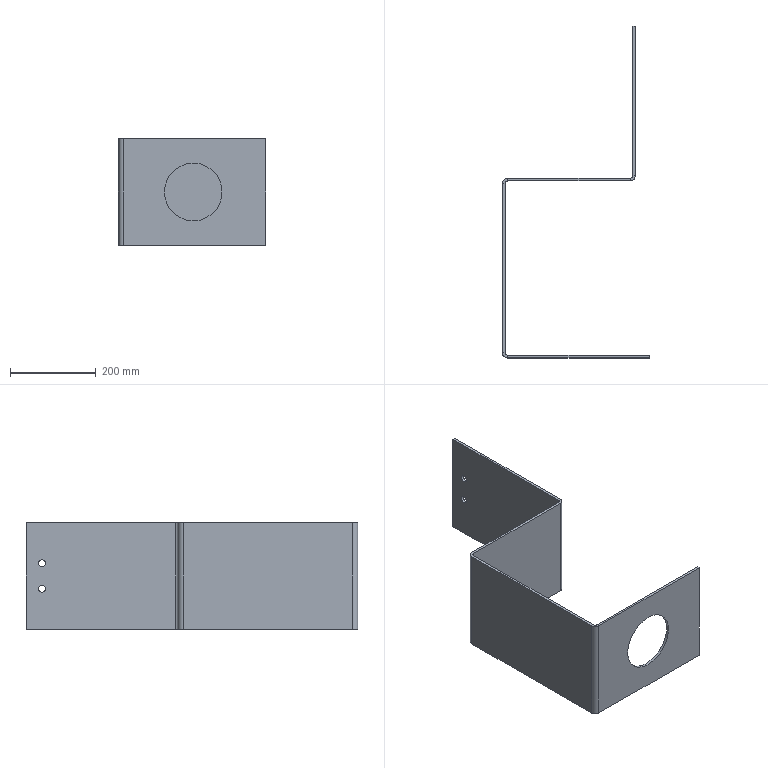Part | SolidWorks | features ICE 2, FlatPattern 1, SMBaseFlange 1, SheetMetal 1 | 1 solid | 36 faces | box 344 x 776 x 250 mm | volume 2022821 mm3 | plane 24 | cylinder 12 | commonest cylinder face diameters 16 x4 12 x3 24 x3 135 x2
STEP:
#1=CARTESIAN_POINT('',(-169.,6.,67.5));
#2=VERTEX_POINT('',#1);
#3=CARTESIAN_POINT('',(-169.,6.,-67.5));
#4=VERTEX_POINT('',#3);
#5=CARTESIAN_POINT('',(-169.,6.,0.));
#6=DIRECTION('',(0.,-1.,0.));
#7=DIRECTION('',(0.,0.,-1.));
#8=AXIS2_PLACEMENT_3D('',#5,#6,#7);
#9=CIRCLE('',#8,67.5);
#10=EDGE_CURVE('',#2,#4,#9,.T.);
#11=ORIENTED_EDGE('',*,*,#10,.F.);
#12=CARTESIAN_POINT('',(-169.,0.,67.5));
#13=VERTEX_POINT('',#12);
#14=CARTESIAN_POINT('',(-169.,6.,67.5));
#15=DIRECTION('',(0.,-1.,0.));
#16=VECTOR('',#15,1000.);
#17=LINE('',#14,#16);
#18=EDGE_CURVE('',#2,#13,#17,.T.);
#19=ORIENTED_EDGE('',*,*,#18,.T.);
#20=CARTESIAN_POINT('',(-169.,0.,-67.5));
#21=VERTEX_POINT('',#20);
#22=CARTESIAN_POINT('',(-169.,0.,0.));
#23=DIRECTION('',(0.,-1.,0.));
#24=DIRECTION('',(0.,0.,-1.));
#25=AXIS2_PLACEMENT_3D('',#22,#23,#24);
#26=CIRCLE('',#25,67.5);
#27=EDGE_CURVE('',#13,#21,#26,.T.);
#28=ORIENTED_EDGE('',*,*,#27,.T.);
#29=CARTESIAN_POINT('',(-169.,6.,-67.5));
#30=DIRECTION('',(0.,-1.,0.));
#31=VECTOR('',#30,1000.);
#32=LINE('',#29,#31);
#33=EDGE_CURVE('',#4,#21,#32,.T.);
#34=ORIENTED_EDGE('',*,*,#33,.F.);
#35=EDGE_LOOP('',(#11,#19,#28,#34));
#36=FACE_OUTER_BOUND('',#35,.T.);
#37=CARTESIAN_POINT('',(-169.,6.,0.));
#38=DIRECTION('',(0.,-1.,0.));
#39=DIRECTION('',(0.,0.,-1.));
#40=AXIS2_PLACEMENT_3D('',#37,#38,#39);
#41=CYLINDRICAL_SURFACE('',#40,67.5);
#42=ADVANCED_FACE('',(#36),#41,.F.);
#43=CARTESIAN_POINT('',(-33.,739.,-38.));
#44=VERTEX_POINT('',#43);
#45=CARTESIAN_POINT('',(-33.,739.,-22.));
#46=VERTEX_POINT('',#45);
#47=CARTESIAN_POINT('',(-33.,739.,-30.));
#48=DIRECTION('',(-1.,0.,0.));
#49=DIRECTION('',(0.,0.,1.));
#50=AXIS2_PLACEMENT_3D('',#47,#48,#49);
#51=CIRCLE('',#50,8.);
#52=EDGE_CURVE('',#44,#46,#51,.T.);
#53=ORIENTED_EDGE('',*,*,#52,.F.);
#54=CARTESIAN_POINT('',(-39.,739.,-38.));
#55=VERTEX_POINT('',#54);
#56=CARTESIAN_POINT('',(-33.,739.,-38.));
#57=DIRECTION('',(-1.,0.,0.));
#58=VECTOR('',#57,1000.);
#59=LINE('',#56,#58);
#60=EDGE_CURVE('',#44,#55,#59,.T.);
#61=ORIENTED_EDGE('',*,*,#60,.T.);
#62=CARTESIAN_POINT('',(-39.,739.,-22.));
#63=VERTEX_POINT('',#62);
#64=CARTESIAN_POINT('',(-39.,739.,-30.));
#65=DIRECTION('',(-1.,0.,0.));
#66=DIRECTION('',(0.,0.,1.));
#67=AXIS2_PLACEMENT_3D('',#64,#65,#66);
#68=CIRCLE('',#67,8.);
#69=EDGE_CURVE('',#55,#63,#68,.T.);
#70=ORIENTED_EDGE('',*,*,#69,.T.);
#71=CARTESIAN_POINT('',(-33.,739.,-22.));
#72=DIRECTION('',(-1.,0.,0.));
#73=VECTOR('',#72,1000.);
#74=LINE('',#71,#73);
#75=EDGE_CURVE('',#46,#63,#74,.T.);
#76=ORIENTED_EDGE('',*,*,#75,.F.);
#77=EDGE_LOOP('',(#53,#61,#70,#76));
#78=FACE_OUTER_BOUND('',#77,.T.);
#79=CARTESIAN_POINT('',(-33.,739.,-30.));
#80=DIRECTION('',(-1.,0.,0.));
#81=DIRECTION('',(0.,0.,1.));
#82=AXIS2_PLACEMENT_3D('',#79,#80,#81);
#83=CYLINDRICAL_SURFACE('',#82,8.);
#84=ADVANCED_FACE('',(#78),#83,.F.);
#85=CARTESIAN_POINT('',(-33.,739.,22.));
#86=VERTEX_POINT('',#85);
#87=CARTESIAN_POINT('',(-33.,739.,38.));
#88=VERTEX_POINT('',#87);
#89=CARTESIAN_POINT('',(-33.,739.,30.));
#90=DIRECTION('',(-1.,0.,0.));
#91=DIRECTION('',(0.,0.,1.));
#92=AXIS2_PLACEMENT_3D('',#89,#90,#91);
#93=CIRCLE('',#92,8.);
#94=EDGE_CURVE('',#86,#88,#93,.T.);
#95=ORIENTED_EDGE('',*,*,#94,.F.);
#96=CARTESIAN_POINT('',(-39.,739.,22.));
#97=VERTEX_POINT('',#96);
#98=CARTESIAN_POINT('',(-33.,739.,22.));
#99=DIRECTION('',(-1.,0.,0.));
#100=VECTOR('',#99,1000.);
#101=LINE('',#98,#100);
#102=EDGE_CURVE('',#86,#97,#101,.T.);
#103=ORIENTED_EDGE('',*,*,#102,.T.);
#104=CARTESIAN_POINT('',(-39.,739.,38.));
#105=VERTEX_POINT('',#104);
#106=CARTESIAN_POINT('',(-39.,739.,30.));
#107=DIRECTION('',(-1.,0.,0.));
#108=DIRECTION('',(0.,0.,1.));
#109=AXIS2_PLACEMENT_3D('',#106,#107,#108);
#110=CIRCLE('',#109,8.);
#111=EDGE_CURVE('',#97,#105,#110,.T.);
#112=ORIENTED_EDGE('',*,*,#111,.T.);
#113=CARTESIAN_POINT('',(-33.,739.,38.));
#114=DIRECTION('',(-1.,0.,0.));
#115=VECTOR('',#114,1000.);
#116=LINE('',#113,#115);
#117=EDGE_CURVE('',#88,#105,#116,.T.);
#118=ORIENTED_EDGE('',*,*,#117,.F.);
#119=EDGE_LOOP('',(#95,#103,#112,#118));
#120=FACE_OUTER_BOUND('',#119,.T.);
#121=CARTESIAN_POINT('',(-33.,739.,30.));
#122=DIRECTION('',(-1.,0.,0.));
#123=DIRECTION('',(0.,0.,1.));
#124=AXIS2_PLACEMENT_3D('',#121,#122,#123);
#125=CYLINDRICAL_SURFACE('',#124,8.);
#126=ADVANCED_FACE('',(#120),#125,.F.);
#127=CARTESIAN_POINT('',(-344.,12.,125.));
#128=VERTEX_POINT('',#127);
#129=CARTESIAN_POINT('',(-338.,12.,125.));
#130=VERTEX_POINT('',#129);
#131=CARTESIAN_POINT('',(-344.,12.,125.));
#132=DIRECTION('',(1.,0.,0.));
#133=VECTOR('',#132,1000.);
#134=LINE('',#131,#133);
#135=EDGE_CURVE('',#128,#130,#134,.T.);
#136=ORIENTED_EDGE('',*,*,#135,.F.);
#137=CARTESIAN_POINT('',(-332.,0.,125.));
#138=VERTEX_POINT('',#137);
#139=CARTESIAN_POINT('',(-332.,12.,125.));
#140=DIRECTION('',(0.,0.,-1.));
#141=DIRECTION('',(1.,0.,0.));
#142=AXIS2_PLACEMENT_3D('',#139,#140,#141);
#143=CIRCLE('',#142,12.);
#144=EDGE_CURVE('',#138,#128,#143,.T.);
#145=ORIENTED_EDGE('',*,*,#144,.F.);
#146=CARTESIAN_POINT('',(-332.,6.,125.));
#147=VERTEX_POINT('',#146);
#148=CARTESIAN_POINT('',(-332.,6.,125.));
#149=DIRECTION('',(0.,-1.,0.));
#150=VECTOR('',#149,1000.);
#151=LINE('',#148,#150);
#152=EDGE_CURVE('',#147,#138,#151,.T.);
#153=ORIENTED_EDGE('',*,*,#152,.F.);
#154=CARTESIAN_POINT('',(-332.,12.,125.));
#155=DIRECTION('',(0.,0.,-1.));
#156=DIRECTION('',(1.,0.,0.));
#157=AXIS2_PLACEMENT_3D('',#154,#155,#156);
#158=CIRCLE('',#157,6.);
#159=EDGE_CURVE('',#147,#130,#158,.T.);
#160=ORIENTED_EDGE('',*,*,#159,.T.);
#161=EDGE_LOOP('',(#136,#145,#153,#160));
#162=FACE_OUTER_BOUND('',#161,.T.);
#163=CARTESIAN_POINT('',(-344.,12.,125.));
#164=DIRECTION('',(0.,0.,1.));
#165=DIRECTION('',(1.,0.,0.));
#166=AXIS2_PLACEMENT_3D('',#163,#164,#165);
#167=PLANE('',#166);
#168=ADVANCED_FACE('',(#162),#167,.T.);
#169=CARTESIAN_POINT('',(-344.,408.,125.));
#170=VERTEX_POINT('',#169);
#171=CARTESIAN_POINT('',(-344.,0.,125.));
#172=DIRECTION('',(0.,1.,0.));
#173=VECTOR('',#172,1000.);
#174=LINE('',#171,#173);
#175=EDGE_CURVE('',#128,#170,#174,.T.);
#176=ORIENTED_EDGE('',*,*,#175,.F.);
#177=ORIENTED_EDGE('',*,*,#135,.T.);
#178=CARTESIAN_POINT('',(-338.,408.,125.));
#179=VERTEX_POINT('',#178);
#180=CARTESIAN_POINT('',(-338.,0.,125.));
#181=DIRECTION('',(0.,1.,0.));
#182=VECTOR('',#181,1000.);
#183=LINE('',#180,#182);
#184=EDGE_CURVE('',#130,#179,#183,.T.);
#185=ORIENTED_EDGE('',*,*,#184,.T.);
#186=CARTESIAN_POINT('',(-338.,408.,125.));
#187=DIRECTION('',(-1.,0.,0.));
#188=VECTOR('',#187,1000.);
#189=LINE('',#186,#188);
#190=EDGE_CURVE('',#179,#170,#189,.T.);
#191=ORIENTED_EDGE('',*,*,#190,.T.);
#192=EDGE_LOOP('',(#176,#177,#185,#191));
#193=FACE_OUTER_BOUND('',#192,.T.);
#194=CARTESIAN_POINT('',(-332.,6.,125.));
#195=DIRECTION('',(0.,0.,1.));
#196=DIRECTION('',(1.,0.,0.));
#197=AXIS2_PLACEMENT_3D('',#194,#195,#196);
#198=PLANE('',#197);
#199=ADVANCED_FACE('',(#193),#198,.T.);
#200=CARTESIAN_POINT('',(-332.,0.,-125.));
#201=VERTEX_POINT('',#200);
#202=CARTESIAN_POINT('',(-332.,6.,-125.));
#203=VERTEX_POINT('',#202);
#204=CARTESIAN_POINT('',(-332.,0.,-125.));
#205=DIRECTION('',(0.,1.,0.));
#206=VECTOR('',#205,1000.);
#207=LINE('',#204,#206);
#208=EDGE_CURVE('',#201,#203,#207,.T.);
#209=ORIENTED_EDGE('',*,*,#208,.F.);
#210=CARTESIAN_POINT('',(-344.,12.,-125.));
#211=VERTEX_POINT('',#210);
#212=CARTESIAN_POINT('',(-332.,12.,-125.));
#213=DIRECTION('',(0.,0.,-1.));
#214=DIRECTION('',(1.,0.,0.));
#215=AXIS2_PLACEMENT_3D('',#212,#213,#214);
#216=CIRCLE('',#215,12.);
#217=EDGE_CURVE('',#201,#211,#216,.T.);
#218=ORIENTED_EDGE('',*,*,#217,.T.);
#219=CARTESIAN_POINT('',(-338.,12.,-125.));
#220=VERTEX_POINT('',#219);
#221=CARTESIAN_POINT('',(-338.,12.,-125.));
#222=DIRECTION('',(-1.,0.,0.));
#223=VECTOR('',#222,1000.);
#224=LINE('',#221,#223);
#225=EDGE_CURVE('',#220,#211,#224,.T.);
#226=ORIENTED_EDGE('',*,*,#225,.F.);
#227=CARTESIAN_POINT('',(-332.,12.,-125.));
#228=DIRECTION('',(0.,0.,-1.));
#229=DIRECTION('',(1.,0.,0.));
#230=AXIS2_PLACEMENT_3D('',#227,#228,#229);
#231=CIRCLE('',#230,6.);
#232=EDGE_CURVE('',#203,#220,#231,.T.);
#233=ORIENTED_EDGE('',*,*,#232,.F.);
#234=EDGE_LOOP('',(#209,#218,#226,#233));
#235=FACE_OUTER_BOUND('',#234,.T.);
#236=CARTESIAN_POINT('',(-332.,0.,-125.));
#237=DIRECTION('',(0.,0.,-1.));
#238=DIRECTION('',(-1.,0.,0.));
#239=AXIS2_PLACEMENT_3D('',#236,#237,#238);
#240=PLANE('',#239);
#241=ADVANCED_FACE('',(#235),#240,.T.);
#242=CARTESIAN_POINT('',(0.,0.,-125.));
#243=VERTEX_POINT('',#242);
#244=CARTESIAN_POINT('',(0.,0.,-125.));
#245=DIRECTION('',(-1.,0.,0.));
#246=VECTOR('',#245,1000.);
#247=LINE('',#244,#246);
#248=EDGE_CURVE('',#243,#201,#247,.T.);
#249=ORIENTED_EDGE('',*,*,#248,.T.);
#250=ORIENTED_EDGE('',*,*,#208,.T.);
#251=CARTESIAN_POINT('',(0.,6.,-125.));
#252=VERTEX_POINT('',#251);
#253=CARTESIAN_POINT('',(0.,6.,-125.));
#254=DIRECTION('',(-1.,0.,0.));
#255=VECTOR('',#254,1000.);
#256=LINE('',#253,#255);
#257=EDGE_CURVE('',#252,#203,#256,.T.);
#258=ORIENTED_EDGE('',*,*,#257,.F.);
#259=CARTESIAN_POINT('',(0.,6.,-125.));
#260=DIRECTION('',(0.,-1.,0.));
#261=VECTOR('',#260,1000.);
#262=LINE('',#259,#261);
#263=EDGE_CURVE('',#252,#243,#262,.T.);
#264=ORIENTED_EDGE('',*,*,#263,.T.);
#265=EDGE_LOOP('',(#249,#250,#258,#264));
#266=FACE_OUTER_BOUND('',#265,.T.);
#267=CARTESIAN_POINT('',(-338.,12.,-125.));
#268=DIRECTION('',(0.,0.,-1.));
#269=DIRECTION('',(-1.,0.,0.));
#270=AXIS2_PLACEMENT_3D('',#267,#268,#269);
#271=PLANE('',#270);
#272=ADVANCED_FACE('',(#266),#271,.T.);
#273=CARTESIAN_POINT('',(-332.,420.,125.));
#274=VERTEX_POINT('',#273);
#275=CARTESIAN_POINT('',(-332.,414.,125.));
#276=VERTEX_POINT('',#275);
#277=CARTESIAN_POINT('',(-332.,420.,125.));
#278=DIRECTION('',(0.,-1.,0.));
#279=VECTOR('',#278,1000.);
#280=LINE('',#277,#279);
#281=EDGE_CURVE('',#274,#276,#280,.T.);
#282=ORIENTED_EDGE('',*,*,#281,.F.);
#283=CARTESIAN_POINT('',(-332.,408.,125.));
#284=DIRECTION('',(0.,0.,-1.));
#285=DIRECTION('',(1.,0.,0.));
#286=AXIS2_PLACEMENT_3D('',#283,#284,#285);
#287=CIRCLE('',#286,12.);
#288=EDGE_CURVE('',#170,#274,#287,.T.);
#289=ORIENTED_EDGE('',*,*,#288,.F.);
#290=ORIENTED_EDGE('',*,*,#190,.F.);
#291=CARTESIAN_POINT('',(-332.,408.,125.));
#292=DIRECTION('',(0.,0.,-1.));
#293=DIRECTION('',(1.,0.,0.));
#294=AXIS2_PLACEMENT_3D('',#291,#292,#293);
#295=CIRCLE('',#294,6.);
#296=EDGE_CURVE('',#179,#276,#295,.T.);
#297=ORIENTED_EDGE('',*,*,#296,.T.);
#298=EDGE_LOOP('',(#282,#289,#290,#297));
#299=FACE_OUTER_BOUND('',#298,.T.);
#300=CARTESIAN_POINT('',(-332.,420.,125.));
#301=DIRECTION('',(0.,0.,1.));
#302=DIRECTION('',(1.,0.,0.));
#303=AXIS2_PLACEMENT_3D('',#300,#301,#302);
#304=PLANE('',#303);
#305=ADVANCED_FACE('',(#299),#304,.T.);
#306=CARTESIAN_POINT('',(-45.,420.,125.));
#307=VERTEX_POINT('',#306);
#308=CARTESIAN_POINT('',(-344.,420.,125.));
#309=DIRECTION('',(1.,0.,0.));
#310=VECTOR('',#309,1000.);
#311=LINE('',#308,#310);
#312=EDGE_CURVE('',#274,#307,#311,.T.);
#313=ORIENTED_EDGE('',*,*,#312,.F.);
#314=ORIENTED_EDGE('',*,*,#281,.T.);
#315=CARTESIAN_POINT('',(-45.,414.,125.));
#316=VERTEX_POINT('',#315);
#317=CARTESIAN_POINT('',(-344.,414.,125.));
#318=DIRECTION('',(1.,0.,0.));
#319=VECTOR('',#318,1000.);
#320=LINE('',#317,#319);
#321=EDGE_CURVE('',#276,#316,#320,.T.);
#322=ORIENTED_EDGE('',*,*,#321,.T.);
#323=CARTESIAN_POINT('',(-45.,414.,125.));
#324=DIRECTION('',(0.,1.,0.));
#325=VECTOR('',#324,1000.);
#326=LINE('',#323,#325);
#327=EDGE_CURVE('',#316,#307,#326,.T.);
#328=ORIENTED_EDGE('',*,*,#327,.T.);
#329=EDGE_LOOP('',(#313,#314,#322,#328));
#330=FACE_OUTER_BOUND('',#329,.T.);
#331=CARTESIAN_POINT('',(-338.,408.,125.));
#332=DIRECTION('',(0.,0.,1.));
#333=DIRECTION('',(1.,0.,0.));
#334=AXIS2_PLACEMENT_3D('',#331,#332,#333);
#335=PLANE('',#334);
#336=ADVANCED_FACE('',(#330),#335,.T.);
#337=CARTESIAN_POINT('',(-344.,408.,-125.));
#338=VERTEX_POINT('',#337);
#339=CARTESIAN_POINT('',(-338.,408.,-125.));
#340=VERTEX_POINT('',#339);
#341=CARTESIAN_POINT('',(-344.,408.,-125.));
#342=DIRECTION('',(1.,0.,0.));
#343=VECTOR('',#342,1000.);
#344=LINE('',#341,#343);
#345=EDGE_CURVE('',#338,#340,#344,.T.);
#346=ORIENTED_EDGE('',*,*,#345,.F.);
#347=CARTESIAN_POINT('',(-332.,420.,-125.));
#348=VERTEX_POINT('',#347);
#349=CARTESIAN_POINT('',(-332.,408.,-125.));
#350=DIRECTION('',(0.,0.,-1.));
#351=DIRECTION('',(1.,0.,0.));
#352=AXIS2_PLACEMENT_3D('',#349,#350,#351);
#353=CIRCLE('',#352,12.);
#354=EDGE_CURVE('',#338,#348,#353,.T.);
#355=ORIENTED_EDGE('',*,*,#354,.T.);
#356=CARTESIAN_POINT('',(-332.,414.,-125.));
#357=VERTEX_POINT('',#356);
#358=CARTESIAN_POINT('',(-332.,414.,-125.));
#359=DIRECTION('',(0.,1.,0.));
#360=VECTOR('',#359,1000.);
#361=LINE('',#358,#360);
#362=EDGE_CURVE('',#357,#348,#361,.T.);
#363=ORIENTED_EDGE('',*,*,#362,.F.);
#364=CARTESIAN_POINT('',(-332.,408.,-125.));
#365=DIRECTION('',(0.,0.,-1.));
#366=DIRECTION('',(1.,0.,0.));
#367=AXIS2_PLACEMENT_3D('',#364,#365,#366);
#368=CIRCLE('',#367,6.);
#369=EDGE_CURVE('',#340,#357,#368,.T.);
#370=ORIENTED_EDGE('',*,*,#369,.F.);
#371=EDGE_LOOP('',(#346,#355,#363,#370));
#372=FACE_OUTER_BOUND('',#371,.T.);
#373=CARTESIAN_POINT('',(-344.,408.,-125.));
#374=DIRECTION('',(0.,0.,-1.));
#375=DIRECTION('',(-1.,0.,0.));
#376=AXIS2_PLACEMENT_3D('',#373,#374,#375);
#377=PLANE('',#376);
#378=ADVANCED_FACE('',(#372),#377,.T.);
#379=CARTESIAN_POINT('',(-344.,0.,-125.));
#380=DIRECTION('',(0.,1.,0.));
#381=VECTOR('',#380,1000.);
#382=LINE('',#379,#381);
#383=EDGE_CURVE('',#211,#338,#382,.T.);
#384=ORIENTED_EDGE('',*,*,#383,.T.);
#385=ORIENTED_EDGE('',*,*,#345,.T.);
#386=CARTESIAN_POINT('',(-338.,0.,-125.));
#387=DIRECTION('',(0.,1.,0.));
#388=VECTOR('',#387,1000.);
#389=LINE('',#386,#388);
#390=EDGE_CURVE('',#220,#340,#389,.T.);
#391=ORIENTED_EDGE('',*,*,#390,.F.);
#392=ORIENTED_EDGE('',*,*,#225,.T.);
#393=EDGE_LOOP('',(#384,#385,#391,#392));
#394=FACE_OUTER_BOUND('',#393,.T.);
#395=CARTESIAN_POINT('',(-332.,414.,-125.));
#396=DIRECTION('',(0.,0.,-1.));
#397=DIRECTION('',(-1.,0.,0.));
#398=AXIS2_PLACEMENT_3D('',#395,#396,#397);
#399=PLANE('',#398);
#400=ADVANCED_FACE('',(#394),#399,.T.);
#401=CARTESIAN_POINT('',(-39.,426.,125.));
#402=VERTEX_POINT('',#401);
#403=CARTESIAN_POINT('',(-33.,426.,125.));
#404=VERTEX_POINT('',#403);
#405=CARTESIAN_POINT('',(-39.,426.,125.));
#406=DIRECTION('',(1.,0.,0.));
#407=VECTOR('',#406,1000.);
#408=LINE('',#405,#407);
#409=EDGE_CURVE('',#402,#404,#408,.T.);
#410=ORIENTED_EDGE('',*,*,#409,.F.);
#411=CARTESIAN_POINT('',(-45.,426.,125.));
#412=DIRECTION('',(0.,0.,1.));
#413=DIRECTION('',(-1.,0.,0.));
#414=AXIS2_PLACEMENT_3D('',#411,#412,#413);
#415=CIRCLE('',#414,6.);
#416=EDGE_CURVE('',#307,#402,#415,.T.);
#417=ORIENTED_EDGE('',*,*,#416,.F.);
#418=ORIENTED_EDGE('',*,*,#327,.F.);
#419=CARTESIAN_POINT('',(-45.,426.,125.));
#420=DIRECTION('',(0.,0.,1.));
#421=DIRECTION('',(1.,0.,0.));
#422=AXIS2_PLACEMENT_3D('',#419,#420,#421);
#423=CIRCLE('',#422,12.);
#424=EDGE_CURVE('',#316,#404,#423,.T.);
#425=ORIENTED_EDGE('',*,*,#424,.T.);
#426=EDGE_LOOP('',(#410,#417,#418,#425));
#427=FACE_OUTER_BOUND('',#426,.T.);
#428=CARTESIAN_POINT('',(-39.,426.,125.));
#429=DIRECTION('',(0.,0.,1.));
#430=DIRECTION('',(1.,0.,0.));
#431=AXIS2_PLACEMENT_3D('',#428,#429,#430);
#432=PLANE('',#431);
#433=ADVANCED_FACE('',(#427),#432,.T.);
#434=CARTESIAN_POINT('',(-39.,776.,125.));
#435=VERTEX_POINT('',#434);
#436=CARTESIAN_POINT('',(-39.,420.,125.));
#437=DIRECTION('',(0.,1.,0.));
#438=VECTOR('',#437,1000.);
#439=LINE('',#436,#438);
#440=EDGE_CURVE('',#402,#435,#439,.T.);
#441=ORIENTED_EDGE('',*,*,#440,.F.);
#442=ORIENTED_EDGE('',*,*,#409,.T.);
#443=CARTESIAN_POINT('',(-33.,776.,125.));
#444=VERTEX_POINT('',#443);
#445=CARTESIAN_POINT('',(-33.,420.,125.));
#446=DIRECTION('',(0.,1.,0.));
#447=VECTOR('',#446,1000.);
#448=LINE('',#445,#447);
#449=EDGE_CURVE('',#404,#444,#448,.T.);
#450=ORIENTED_EDGE('',*,*,#449,.T.);
#451=CARTESIAN_POINT('',(-39.,776.,125.));
#452=DIRECTION('',(1.,0.,0.));
#453=VECTOR('',#452,1000.);
#454=LINE('',#451,#453);
#455=EDGE_CURVE('',#435,#444,#454,.T.);
#456=ORIENTED_EDGE('',*,*,#455,.F.);
#457=EDGE_LOOP('',(#441,#442,#450,#456));
#458=FACE_OUTER_BOUND('',#457,.T.);
#459=CARTESIAN_POINT('',(-45.,414.,125.));
#460=DIRECTION('',(0.,0.,1.));
#461=DIRECTION('',(1.,0.,0.));
#462=AXIS2_PLACEMENT_3D('',#459,#460,#461);
#463=PLANE('',#462);
#464=ADVANCED_FACE('',(#458),#463,.T.);
#465=CARTESIAN_POINT('',(-45.,420.,-125.));
#466=VERTEX_POINT('',#465);
#467=CARTESIAN_POINT('',(-45.,414.,-125.));
#468=VERTEX_POINT('',#467);
#469=CARTESIAN_POINT('',(-45.,420.,-125.));
#470=DIRECTION('',(0.,-1.,0.));
#471=VECTOR('',#470,1000.);
#472=LINE('',#469,#471);
#473=EDGE_CURVE('',#466,#468,#472,.T.);
#474=ORIENTED_EDGE('',*,*,#473,.F.);
#475=CARTESIAN_POINT('',(-39.,426.,-125.));
#476=VERTEX_POINT('',#475);
#477=CARTESIAN_POINT('',(-45.,426.,-125.));
#478=DIRECTION('',(0.,0.,1.));
#479=DIRECTION('',(-1.,0.,0.));
#480=AXIS2_PLACEMENT_3D('',#477,#478,#479);
#481=CIRCLE('',#480,6.);
#482=EDGE_CURVE('',#466,#476,#481,.T.);
#483=ORIENTED_EDGE('',*,*,#482,.T.);
#484=CARTESIAN_POINT('',(-33.,426.,-125.));
#485=VERTEX_POINT('',#484);
#486=CARTESIAN_POINT('',(-33.,426.,-125.));
#487=DIRECTION('',(-1.,0.,0.));
#488=VECTOR('',#487,1000.);
#489=LINE('',#486,#488);
#490=EDGE_CURVE('',#485,#476,#489,.T.);
#491=ORIENTED_EDGE('',*,*,#490,.F.);
#492=CARTESIAN_POINT('',(-45.,426.,-125.));
#493=DIRECTION('',(0.,0.,1.));
#494=DIRECTION('',(1.,0.,0.));
#495=AXIS2_PLACEMENT_3D('',#492,#493,#494);
#496=CIRCLE('',#495,12.);
#497=EDGE_CURVE('',#468,#485,#496,.T.);
#498=ORIENTED_EDGE('',*,*,#497,.F.);
#499=EDGE_LOOP('',(#474,#483,#491,#498));
#500=FACE_OUTER_BOUND('',#499,.T.);
#501=CARTESIAN_POINT('',(-45.,420.,-125.));
#502=DIRECTION('',(0.,0.,-1.));
#503=DIRECTION('',(-1.,0.,0.));
#504=AXIS2_PLACEMENT_3D('',#501,#502,#503);
#505=PLANE('',#504);
#506=ADVANCED_FACE('',(#500),#505,.T.);
#507=CARTESIAN_POINT('',(-344.,420.,-125.));
#508=DIRECTION('',(1.,0.,0.));
#509=VECTOR('',#508,1000.);
#510=LINE('',#507,#509);
#511=EDGE_CURVE('',#348,#466,#510,.T.);
#512=ORIENTED_EDGE('',*,*,#511,.T.);
#513=ORIENTED_EDGE('',*,*,#473,.T.);
#514=CARTESIAN_POINT('',(-344.,414.,-125.));
#515=DIRECTION('',(1.,0.,0.));
#516=VECTOR('',#515,1000.);
#517=LINE('',#514,#516);
#518=EDGE_CURVE('',#357,#468,#517,.T.);
#519=ORIENTED_EDGE('',*,*,#518,.F.);
#520=ORIENTED_EDGE('',*,*,#362,.T.);
#521=EDGE_LOOP('',(#512,#513,#519,#520));
#522=FACE_OUTER_BOUND('',#521,.T.);
#523=CARTESIAN_POINT('',(-33.,426.,-125.));
#524=DIRECTION('',(0.,0.,-1.));
#525=DIRECTION('',(-1.,0.,0.));
#526=AXIS2_PLACEMENT_3D('',#523,#524,#525);
#527=PLANE('',#526);
#528=ADVANCED_FACE('',(#522),#527,.T.);
#529=CARTESIAN_POINT('',(-33.,739.,-30.));
#530=DIRECTION('',(-1.,0.,0.));
#531=DIRECTION('',(0.,0.,1.));
#532=AXIS2_PLACEMENT_3D('',#529,#530,#531);
#533=CIRCLE('',#532,8.);
#534=EDGE_CURVE('',#46,#44,#533,.T.);
#535=ORIENTED_EDGE('',*,*,#534,.T.);
#536=ORIENTED_EDGE('',*,*,#52,.T.);
#537=EDGE_LOOP('',(#535,#536));
#538=FACE_BOUND('',#537,.T.);
#539=CARTESIAN_POINT('',(-33.,739.,30.));
#540=DIRECTION('',(-1.,0.,0.));
#541=DIRECTION('',(0.,0.,1.));
#542=AXIS2_PLACEMENT_3D('',#539,#540,#541);
#543=CIRCLE('',#542,8.);
#544=EDGE_CURVE('',#88,#86,#543,.T.);
#545=ORIENTED_EDGE('',*,*,#544,.T.);
#546=ORIENTED_EDGE('',*,*,#94,.T.);
#547=EDGE_LOOP('',(#545,#546));
#548=FACE_BOUND('',#547,.T.);
#549=CARTESIAN_POINT('',(-33.,776.,-125.));
#550=VERTEX_POINT('',#549);
#551=CARTESIAN_POINT('',(-33.,420.,-125.));
#552=DIRECTION('',(0.,1.,0.));
#553=VECTOR('',#552,1000.);
#554=LINE('',#551,#553);
#555=EDGE_CURVE('',#485,#550,#554,.T.);
#556=ORIENTED_EDGE('',*,*,#555,.T.);
#557=CARTESIAN_POINT('',(-33.,776.,125.));
#558=DIRECTION('',(0.,0.,-1.));
#559=VECTOR('',#558,1000.);
#560=LINE('',#557,#559);
#561=EDGE_CURVE('',#444,#550,#560,.T.);
#562=ORIENTED_EDGE('',*,*,#561,.F.);
#563=ORIENTED_EDGE('',*,*,#449,.F.);
#564=CARTESIAN_POINT('',(-33.,426.,125.));
#565=DIRECTION('',(0.,0.,-1.));
#566=VECTOR('',#565,1000.);
#567=LINE('',#564,#566);
#568=EDGE_CURVE('',#404,#485,#567,.T.);
#569=ORIENTED_EDGE('',*,*,#568,.T.);
#570=EDGE_LOOP('',(#556,#562,#563,#569));
#571=FACE_OUTER_BOUND('',#570,.T.);
#572=CARTESIAN_POINT('',(-33.,420.,125.));
#573=DIRECTION('',(-1.,0.,0.));
#574=DIRECTION('',(0.,0.,1.));
#575=AXIS2_PLACEMENT_3D('',#572,#573,#574);
#576=PLANE('',#575);
#577=ADVANCED_FACE('',(#538,#548,#571),#576,.F.);
#578=CARTESIAN_POINT('',(-39.,776.,-125.));
#579=VERTEX_POINT('',#578);
#580=CARTESIAN_POINT('',(-39.,776.,-125.));
#581=DIRECTION('',(1.,0.,0.));
#582=VECTOR('',#581,1000.);
#583=LINE('',#580,#582);
#584=EDGE_CURVE('',#579,#550,#583,.T.);
#585=ORIENTED_EDGE('',*,*,#584,.F.);
#586=CARTESIAN_POINT('',(-39.,776.,125.));
#587=DIRECTION('',(0.,0.,-1.));
#588=VECTOR('',#587,1000.);
#589=LINE('',#586,#588);
#590=EDGE_CURVE('',#435,#579,#589,.T.);
#591=ORIENTED_EDGE('',*,*,#590,.F.);
#592=ORIENTED_EDGE('',*,*,#455,.T.);
#593=ORIENTED_EDGE('',*,*,#561,.T.);
#594=EDGE_LOOP('',(#585,#591,#592,#593));
#595=FACE_OUTER_BOUND('',#594,.T.);
#596=CARTESIAN_POINT('',(-39.,776.,125.));
#597=DIRECTION('',(0.,1.,0.));
#598=DIRECTION('',(0.,0.,1.));
#599=AXIS2_PLACEMENT_3D('',#596,#597,#598);
#600=PLANE('',#599);
#601=ADVANCED_FACE('',(#595),#600,.T.);
#602=CARTESIAN_POINT('',(-39.,739.,-30.));
#603=DIRECTION('',(-1.,0.,0.));
#604=DIRECTION('',(0.,0.,1.));
#605=AXIS2_PLACEMENT_3D('',#602,#603,#604);
#606=CIRCLE('',#605,8.);
#607=EDGE_CURVE('',#63,#55,#606,.T.);
#608=ORIENTED_EDGE('',*,*,#607,.F.);
#609=ORIENTED_EDGE('',*,*,#69,.F.);
#610=EDGE_LOOP('',(#608,#609));
#611=FACE_BOUND('',#610,.T.);
#612=CARTESIAN_POINT('',(-39.,739.,30.));
#613=DIRECTION('',(-1.,0.,0.));
#614=DIRECTION('',(0.,0.,1.));
#615=AXIS2_PLACEMENT_3D('',#612,#613,#614);
#616=CIRCLE('',#615,8.);
#617=EDGE_CURVE('',#105,#97,#616,.T.);
#618=ORIENTED_EDGE('',*,*,#617,.F.);
#619=ORIENTED_EDGE('',*,*,#111,.F.);
#620=EDGE_LOOP('',(#618,#619));
#621=FACE_BOUND('',#620,.T.);
#622=CARTESIAN_POINT('',(-39.,420.,-125.));
#623=DIRECTION('',(0.,1.,0.));
#624=VECTOR('',#623,1000.);
#625=LINE('',#622,#624);
#626=EDGE_CURVE('',#476,#579,#625,.T.);
#627=ORIENTED_EDGE('',*,*,#626,.F.);
#628=CARTESIAN_POINT('',(-39.,426.,125.));
#629=DIRECTION('',(0.,0.,-1.));
#630=VECTOR('',#629,1000.);
#631=LINE('',#628,#630);
#632=EDGE_CURVE('',#402,#476,#631,.T.);
#633=ORIENTED_EDGE('',*,*,#632,.F.);
#634=ORIENTED_EDGE('',*,*,#440,.T.);
#635=ORIENTED_EDGE('',*,*,#590,.T.);
#636=EDGE_LOOP('',(#627,#633,#634,#635));
#637=FACE_OUTER_BOUND('',#636,.T.);
#638=CARTESIAN_POINT('',(-39.,420.,125.));
#639=DIRECTION('',(-1.,0.,0.));
#640=DIRECTION('',(0.,0.,1.));
#641=AXIS2_PLACEMENT_3D('',#638,#639,#640);
#642=PLANE('',#641);
#643=ADVANCED_FACE('',(#611,#621,#637),#642,.T.);
#644=ORIENTED_EDGE('',*,*,#482,.F.);
#645=CARTESIAN_POINT('',(-45.,420.,125.));
#646=DIRECTION('',(0.,0.,-1.));
#647=VECTOR('',#646,1000.);
#648=LINE('',#645,#647);
#649=EDGE_CURVE('',#307,#466,#648,.T.);
#650=ORIENTED_EDGE('',*,*,#649,.F.);
#651=ORIENTED_EDGE('',*,*,#416,.T.);
#652=ORIENTED_EDGE('',*,*,#632,.T.);
#653=EDGE_LOOP('',(#644,#650,#651,#652));
#654=FACE_OUTER_BOUND('',#653,.T.);
#655=CARTESIAN_POINT('',(-45.,426.,125.));
#656=DIRECTION('',(0.,0.,-1.));
#657=DIRECTION('',(-1.,0.,0.));
#658=AXIS2_PLACEMENT_3D('',#655,#656,#657);
#659=CYLINDRICAL_SURFACE('',#658,6.);
#660=ADVANCED_FACE('',(#654),#659,.F.);
#661=ORIENTED_EDGE('',*,*,#511,.F.);
#662=CARTESIAN_POINT('',(-332.,420.,125.));
#663=DIRECTION('',(0.,0.,-1.));
#664=VECTOR('',#663,1000.);
#665=LINE('',#662,#664);
#666=EDGE_CURVE('',#274,#348,#665,.T.);
#667=ORIENTED_EDGE('',*,*,#666,.F.);
#668=ORIENTED_EDGE('',*,*,#312,.T.);
#669=ORIENTED_EDGE('',*,*,#649,.T.);
#670=EDGE_LOOP('',(#661,#667,#668,#669));
#671=FACE_OUTER_BOUND('',#670,.T.);
#672=CARTESIAN_POINT('',(-344.,420.,125.));
#673=DIRECTION('',(0.,1.,0.));
#674=DIRECTION('',(0.,0.,1.));
#675=AXIS2_PLACEMENT_3D('',#672,#673,#674);
#676=PLANE('',#675);
#677=ADVANCED_FACE('',(#671),#676,.T.);
#678=ORIENTED_EDGE('',*,*,#354,.F.);
#679=CARTESIAN_POINT('',(-344.,408.,125.));
#680=DIRECTION('',(0.,0.,-1.));
#681=VECTOR('',#680,1000.);
#682=LINE('',#679,#681);
#683=EDGE_CURVE('',#170,#338,#682,.T.);
#684=ORIENTED_EDGE('',*,*,#683,.F.);
#685=ORIENTED_EDGE('',*,*,#288,.T.);
#686=ORIENTED_EDGE('',*,*,#666,.T.);
#687=EDGE_LOOP('',(#678,#684,#685,#686));
#688=FACE_OUTER_BOUND('',#687,.T.);
#689=CARTESIAN_POINT('',(-332.,408.,125.));
#690=DIRECTION('',(0.,0.,-1.));
#691=DIRECTION('',(-1.,0.,0.));
#692=AXIS2_PLACEMENT_3D('',#689,#690,#691);
#693=CYLINDRICAL_SURFACE('',#692,12.);
#694=ADVANCED_FACE('',(#688),#693,.T.);
#695=ORIENTED_EDGE('',*,*,#383,.F.);
#696=CARTESIAN_POINT('',(-344.,12.,125.));
#697=DIRECTION('',(0.,0.,-1.));
#698=VECTOR('',#697,1000.);
#699=LINE('',#696,#698);
#700=EDGE_CURVE('',#128,#211,#699,.T.);
#701=ORIENTED_EDGE('',*,*,#700,.F.);
#702=ORIENTED_EDGE('',*,*,#175,.T.);
#703=ORIENTED_EDGE('',*,*,#683,.T.);
#704=EDGE_LOOP('',(#695,#701,#702,#703));
#705=FACE_OUTER_BOUND('',#704,.T.);
#706=CARTESIAN_POINT('',(-344.,0.,125.));
#707=DIRECTION('',(-1.,0.,0.));
#708=DIRECTION('',(0.,0.,1.));
#709=AXIS2_PLACEMENT_3D('',#706,#707,#708);
#710=PLANE('',#709);
#711=ADVANCED_FACE('',(#705),#710,.T.);
#712=ORIENTED_EDGE('',*,*,#217,.F.);
#713=CARTESIAN_POINT('',(-332.,0.,125.));
#714=DIRECTION('',(0.,0.,-1.));
#715=VECTOR('',#714,1000.);
#716=LINE('',#713,#715);
#717=EDGE_CURVE('',#138,#201,#716,.T.);
#718=ORIENTED_EDGE('',*,*,#717,.F.);
#719=ORIENTED_EDGE('',*,*,#144,.T.);
#720=ORIENTED_EDGE('',*,*,#700,.T.);
#721=EDGE_LOOP('',(#712,#718,#719,#720));
#722=FACE_OUTER_BOUND('',#721,.T.);
#723=CARTESIAN_POINT('',(-332.,12.,125.));
#724=DIRECTION('',(0.,0.,-1.));
#725=DIRECTION('',(-1.,0.,0.));
#726=AXIS2_PLACEMENT_3D('',#723,#724,#725);
#727=CYLINDRICAL_SURFACE('',#726,12.);
#728=ADVANCED_FACE('',(#722),#727,.T.);
#729=CARTESIAN_POINT('',(-169.,0.,0.));
#730=DIRECTION('',(0.,-1.,0.));
#731=DIRECTION('',(0.,0.,-1.));
#732=AXIS2_PLACEMENT_3D('',#729,#730,#731);
#733=CIRCLE('',#732,67.5);
#734=EDGE_CURVE('',#21,#13,#733,.T.);
#735=ORIENTED_EDGE('',*,*,#734,.F.);
#736=ORIENTED_EDGE('',*,*,#27,.F.);
#737=EDGE_LOOP('',(#735,#736));
#738=FACE_BOUND('',#737,.T.);
#739=ORIENTED_EDGE('',*,*,#248,.F.);
#740=CARTESIAN_POINT('',(0.,0.,125.));
#741=VERTEX_POINT('',#740);
#742=CARTESIAN_POINT('',(0.,0.,125.));
#743=DIRECTION('',(0.,0.,-1.));
#744=VECTOR('',#743,1000.);
#745=LINE('',#742,#744);
#746=EDGE_CURVE('',#741,#243,#745,.T.);
#747=ORIENTED_EDGE('',*,*,#746,.F.);
#748=CARTESIAN_POINT('',(0.,0.,125.));
#749=DIRECTION('',(-1.,0.,0.));
#750=VECTOR('',#749,1000.);
#751=LINE('',#748,#750);
#752=EDGE_CURVE('',#741,#138,#751,.T.);
#753=ORIENTED_EDGE('',*,*,#752,.T.);
#754=ORIENTED_EDGE('',*,*,#717,.T.);
#755=EDGE_LOOP('',(#739,#747,#753,#754));
#756=FACE_OUTER_BOUND('',#755,.T.);
#757=CARTESIAN_POINT('',(0.,0.,125.));
#758=DIRECTION('',(0.,-1.,0.));
#759=DIRECTION('',(0.,0.,-1.));
#760=AXIS2_PLACEMENT_3D('',#757,#758,#759);
#761=PLANE('',#760);
#762=ADVANCED_FACE('',(#738,#756),#761,.T.);
#763=ORIENTED_EDGE('',*,*,#263,.F.);
#764=CARTESIAN_POINT('',(0.,6.,125.));
#765=VERTEX_POINT('',#764);
#766=CARTESIAN_POINT('',(0.,6.,125.));
#767=DIRECTION('',(0.,0.,-1.));
#768=VECTOR('',#767,1000.);
#769=LINE('',#766,#768);
#770=EDGE_CURVE('',#765,#252,#769,.T.);
#771=ORIENTED_EDGE('',*,*,#770,.F.);
#772=CARTESIAN_POINT('',(0.,6.,125.));
#773=DIRECTION('',(0.,-1.,0.));
#774=VECTOR('',#773,1000.);
#775=LINE('',#772,#774);
#776=EDGE_CURVE('',#765,#741,#775,.T.);
#777=ORIENTED_EDGE('',*,*,#776,.T.);
#778=ORIENTED_EDGE('',*,*,#746,.T.);
#779=EDGE_LOOP('',(#763,#771,#777,#778));
#780=FACE_OUTER_BOUND('',#779,.T.);
#781=CARTESIAN_POINT('',(0.,6.,125.));
#782=DIRECTION('',(1.,0.,0.));
#783=DIRECTION('',(0.,0.,-1.));
#784=AXIS2_PLACEMENT_3D('',#781,#782,#783);
#785=PLANE('',#784);
#786=ADVANCED_FACE('',(#780),#785,.T.);
#787=CARTESIAN_POINT('',(-169.,6.,0.));
#788=DIRECTION('',(0.,-1.,0.));
#789=DIRECTION('',(0.,0.,-1.));
#790=AXIS2_PLACEMENT_3D('',#787,#788,#789);
#791=CIRCLE('',#790,67.5);
#792=EDGE_CURVE('',#4,#2,#791,.T.);
#793=ORIENTED_EDGE('',*,*,#792,.T.);
#794=ORIENTED_EDGE('',*,*,#10,.T.);
#795=EDGE_LOOP('',(#793,#794));
#796=FACE_BOUND('',#795,.T.);
#797=ORIENTED_EDGE('',*,*,#257,.T.);
#798=CARTESIAN_POINT('',(-332.,6.,125.));
#799=DIRECTION('',(0.,0.,-1.));
#800=VECTOR('',#799,1000.);
#801=LINE('',#798,#800);
#802=EDGE_CURVE('',#147,#203,#801,.T.);
#803=ORIENTED_EDGE('',*,*,#802,.F.);
#804=CARTESIAN_POINT('',(0.,6.,125.));
#805=DIRECTION('',(-1.,0.,0.));
#806=VECTOR('',#805,1000.);
#807=LINE('',#804,#806);
#808=EDGE_CURVE('',#765,#147,#807,.T.);
#809=ORIENTED_EDGE('',*,*,#808,.F.);
#810=ORIENTED_EDGE('',*,*,#770,.T.);
#811=EDGE_LOOP('',(#797,#803,#809,#810));
#812=FACE_OUTER_BOUND('',#811,.T.);
#813=CARTESIAN_POINT('',(0.,6.,125.));
#814=DIRECTION('',(0.,-1.,0.));
#815=DIRECTION('',(0.,0.,-1.));
#816=AXIS2_PLACEMENT_3D('',#813,#814,#815);
#817=PLANE('',#816);
#818=ADVANCED_FACE('',(#796,#812),#817,.F.);
#819=ORIENTED_EDGE('',*,*,#232,.T.);
#820=CARTESIAN_POINT('',(-338.,12.,125.));
#821=DIRECTION('',(0.,0.,-1.));
#822=VECTOR('',#821,1000.);
#823=LINE('',#820,#822);
#824=EDGE_CURVE('',#130,#220,#823,.T.);
#825=ORIENTED_EDGE('',*,*,#824,.F.);
#826=ORIENTED_EDGE('',*,*,#159,.F.);
#827=ORIENTED_EDGE('',*,*,#802,.T.);
#828=EDGE_LOOP('',(#819,#825,#826,#827));
#829=FACE_OUTER_BOUND('',#828,.T.);
#830=CARTESIAN_POINT('',(-332.,12.,125.));
#831=DIRECTION('',(0.,0.,-1.));
#832=DIRECTION('',(-1.,0.,0.));
#833=AXIS2_PLACEMENT_3D('',#830,#831,#832);
#834=CYLINDRICAL_SURFACE('',#833,6.);
#835=ADVANCED_FACE('',(#829),#834,.F.);
#836=ORIENTED_EDGE('',*,*,#390,.T.);
#837=CARTESIAN_POINT('',(-338.,408.,125.));
#838=DIRECTION('',(0.,0.,-1.));
#839=VECTOR('',#838,1000.);
#840=LINE('',#837,#839);
#841=EDGE_CURVE('',#179,#340,#840,.T.);
#842=ORIENTED_EDGE('',*,*,#841,.F.);
#843=ORIENTED_EDGE('',*,*,#184,.F.);
#844=ORIENTED_EDGE('',*,*,#824,.T.);
#845=EDGE_LOOP('',(#836,#842,#843,#844));
#846=FACE_OUTER_BOUND('',#845,.T.);
#847=CARTESIAN_POINT('',(-338.,0.,125.));
#848=DIRECTION('',(-1.,0.,0.));
#849=DIRECTION('',(0.,0.,1.));
#850=AXIS2_PLACEMENT_3D('',#847,#848,#849);
#851=PLANE('',#850);
#852=ADVANCED_FACE('',(#846),#851,.F.);
#853=ORIENTED_EDGE('',*,*,#369,.T.);
#854=CARTESIAN_POINT('',(-332.,414.,125.));
#855=DIRECTION('',(0.,0.,-1.));
#856=VECTOR('',#855,1000.);
#857=LINE('',#854,#856);
#858=EDGE_CURVE('',#276,#357,#857,.T.);
#859=ORIENTED_EDGE('',*,*,#858,.F.);
#860=ORIENTED_EDGE('',*,*,#296,.F.);
#861=ORIENTED_EDGE('',*,*,#841,.T.);
#862=EDGE_LOOP('',(#853,#859,#860,#861));
#863=FACE_OUTER_BOUND('',#862,.T.);
#864=CARTESIAN_POINT('',(-332.,408.,125.));
#865=DIRECTION('',(0.,0.,-1.));
#866=DIRECTION('',(-1.,0.,0.));
#867=AXIS2_PLACEMENT_3D('',#864,#865,#866);
#868=CYLINDRICAL_SURFACE('',#867,6.);
#869=ADVANCED_FACE('',(#863),#868,.F.);
#870=ORIENTED_EDGE('',*,*,#518,.T.);
#871=CARTESIAN_POINT('',(-45.,414.,125.));
#872=DIRECTION('',(0.,0.,-1.));
#873=VECTOR('',#872,1000.);
#874=LINE('',#871,#873);
#875=EDGE_CURVE('',#316,#468,#874,.T.);
#876=ORIENTED_EDGE('',*,*,#875,.F.);
#877=ORIENTED_EDGE('',*,*,#321,.F.);
#878=ORIENTED_EDGE('',*,*,#858,.T.);
#879=EDGE_LOOP('',(#870,#876,#877,#878));
#880=FACE_OUTER_BOUND('',#879,.T.);
#881=CARTESIAN_POINT('',(-344.,414.,125.));
#882=DIRECTION('',(0.,1.,0.));
#883=DIRECTION('',(0.,0.,1.));
#884=AXIS2_PLACEMENT_3D('',#881,#882,#883);
#885=PLANE('',#884);
#886=ADVANCED_FACE('',(#880),#885,.F.);
#887=ORIENTED_EDGE('',*,*,#497,.T.);
#888=ORIENTED_EDGE('',*,*,#568,.F.);
#889=ORIENTED_EDGE('',*,*,#424,.F.);
#890=ORIENTED_EDGE('',*,*,#875,.T.);
#891=EDGE_LOOP('',(#887,#888,#889,#890));
#892=FACE_OUTER_BOUND('',#891,.T.);
#893=CARTESIAN_POINT('',(-45.,426.,125.));
#894=DIRECTION('',(0.,0.,-1.));
#895=DIRECTION('',(-1.,0.,0.));
#896=AXIS2_PLACEMENT_3D('',#893,#894,#895);
#897=CYLINDRICAL_SURFACE('',#896,12.);
#898=ADVANCED_FACE('',(#892),#897,.T.);
#899=ORIENTED_EDGE('',*,*,#808,.T.);
#900=ORIENTED_EDGE('',*,*,#152,.T.);
#901=ORIENTED_EDGE('',*,*,#752,.F.);
#902=ORIENTED_EDGE('',*,*,#776,.F.);
#903=EDGE_LOOP('',(#899,#900,#901,#902));
#904=FACE_OUTER_BOUND('',#903,.T.);
#905=CARTESIAN_POINT('',(-45.,426.,125.));
#906=DIRECTION('',(0.,0.,-1.));
#907=DIRECTION('',(-1.,0.,0.));
#908=AXIS2_PLACEMENT_3D('',#905,#906,#907);
#909=PLANE('',#908);
#910=ADVANCED_FACE('',(#904),#909,.F.);
#911=ORIENTED_EDGE('',*,*,#555,.F.);
#912=ORIENTED_EDGE('',*,*,#490,.T.);
#913=ORIENTED_EDGE('',*,*,#626,.T.);
#914=ORIENTED_EDGE('',*,*,#584,.T.);
#915=EDGE_LOOP('',(#911,#912,#913,#914));
#916=FACE_OUTER_BOUND('',#915,.T.);
#917=CARTESIAN_POINT('',(-45.,426.,-125.));
#918=DIRECTION('',(0.,0.,-1.));
#919=DIRECTION('',(-1.,0.,0.));
#920=AXIS2_PLACEMENT_3D('',#917,#918,#919);
#921=PLANE('',#920);
#922=ADVANCED_FACE('',(#916),#921,.T.);
#923=ORIENTED_EDGE('',*,*,#102,.F.);
#924=ORIENTED_EDGE('',*,*,#544,.F.);
#925=ORIENTED_EDGE('',*,*,#117,.T.);
#926=ORIENTED_EDGE('',*,*,#617,.T.);
#927=EDGE_LOOP('',(#923,#924,#925,#926));
#928=FACE_OUTER_BOUND('',#927,.T.);
#929=CARTESIAN_POINT('',(-33.,739.,30.));
#930=DIRECTION('',(-1.,0.,0.));
#931=DIRECTION('',(0.,0.,1.));
#932=AXIS2_PLACEMENT_3D('',#929,#930,#931);
#933=CYLINDRICAL_SURFACE('',#932,8.);
#934=ADVANCED_FACE('',(#928),#933,.F.);
#935=ORIENTED_EDGE('',*,*,#60,.F.);
#936=ORIENTED_EDGE('',*,*,#534,.F.);
#937=ORIENTED_EDGE('',*,*,#75,.T.);
#938=ORIENTED_EDGE('',*,*,#607,.T.);
#939=EDGE_LOOP('',(#935,#936,#937,#938));
#940=FACE_OUTER_BOUND('',#939,.T.);
#941=CARTESIAN_POINT('',(-33.,739.,-30.));
#942=DIRECTION('',(-1.,0.,0.));
#943=DIRECTION('',(0.,0.,1.));
#944=AXIS2_PLACEMENT_3D('',#941,#942,#943);
#945=CYLINDRICAL_SURFACE('',#944,8.);
#946=ADVANCED_FACE('',(#940),#945,.F.);
#947=ORIENTED_EDGE('',*,*,#18,.F.);
#948=ORIENTED_EDGE('',*,*,#792,.F.);
#949=ORIENTED_EDGE('',*,*,#33,.T.);
#950=ORIENTED_EDGE('',*,*,#734,.T.);
#951=EDGE_LOOP('',(#947,#948,#949,#950));
#952=FACE_OUTER_BOUND('',#951,.T.);
#953=CARTESIAN_POINT('',(-169.,6.,0.));
#954=DIRECTION('',(0.,-1.,0.));
#955=DIRECTION('',(0.,0.,-1.));
#956=AXIS2_PLACEMENT_3D('',#953,#954,#955);
#957=CYLINDRICAL_SURFACE('',#956,67.5);
#958=ADVANCED_FACE('',(#952),#957,.F.);
#959=CLOSED_SHELL('',(#42,#84,#126,#168,#199,#241,#272,#305,#336,#378,#400,#433,#464,#506,#528,#577,#601,#643,#660,#677,#694,#711,#728,#762,#786,#818,#835,#852,#869,#886,#898,#910,#922,#934,#946,#958));
#960=MANIFOLD_SOLID_BREP('',#959);
#961=CARTESIAN_POINT('',(0.,0.,0.));
#962=DIRECTION('',(0.,0.,1.));
#963=DIRECTION('',(1.,0.,0.));
#964=AXIS2_PLACEMENT_3D('',#961,#962,#963);
#965=(LENGTH_UNIT()NAMED_UNIT(*)SI_UNIT(.MILLI.,.METRE.));
#966=UNCERTAINTY_MEASURE_WITH_UNIT(LENGTH_MEASURE(0.00001),#965,'','');
#967=(NAMED_UNIT(*)PLANE_ANGLE_UNIT()SI_UNIT($,.RADIAN.));
#968=(NAMED_UNIT(*)SI_UNIT($,.STERADIAN.)SOLID_ANGLE_UNIT());
#969=(GEOMETRIC_REPRESENTATION_CONTEXT(3)GLOBAL_UNCERTAINTY_ASSIGNED_CONTEXT((#966))GLOBAL_UNIT_ASSIGNED_CONTEXT((#965,#967,#968))REPRESENTATION_CONTEXT('',''));
#970=ADVANCED_BREP_SHAPE_REPRESENTATION('',(#960,#964),#969);